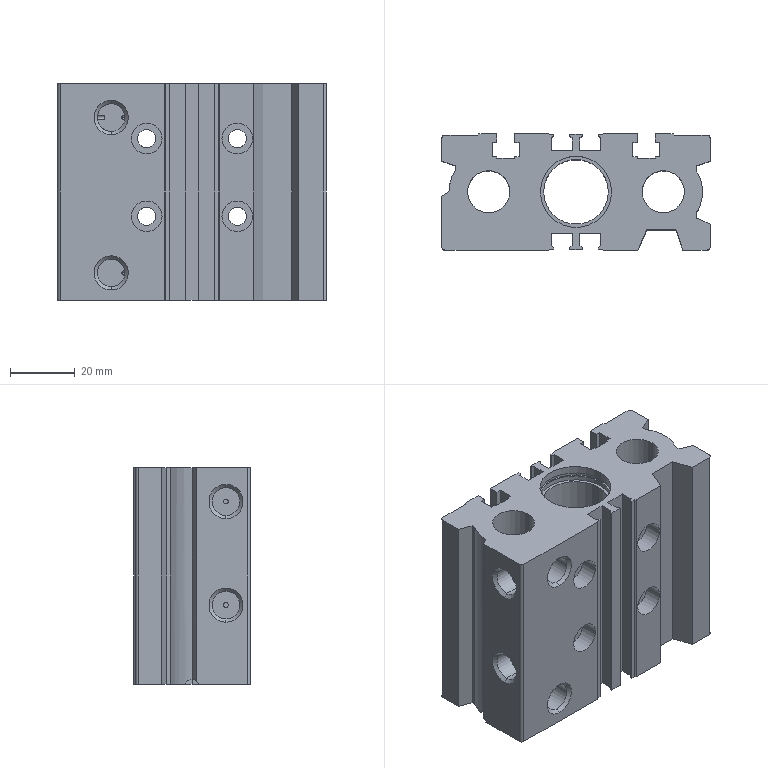Part | 1 solid | 230 faces | box 83 x 36 x 67 mm | volume 125239 mm3 | plane 107 | cylinder 83 | cone 40 | commonest cylinder face diameters 1.5 x8 3 x8 3.5 x8 4.2 x8 5.6 x8 8.566 x8